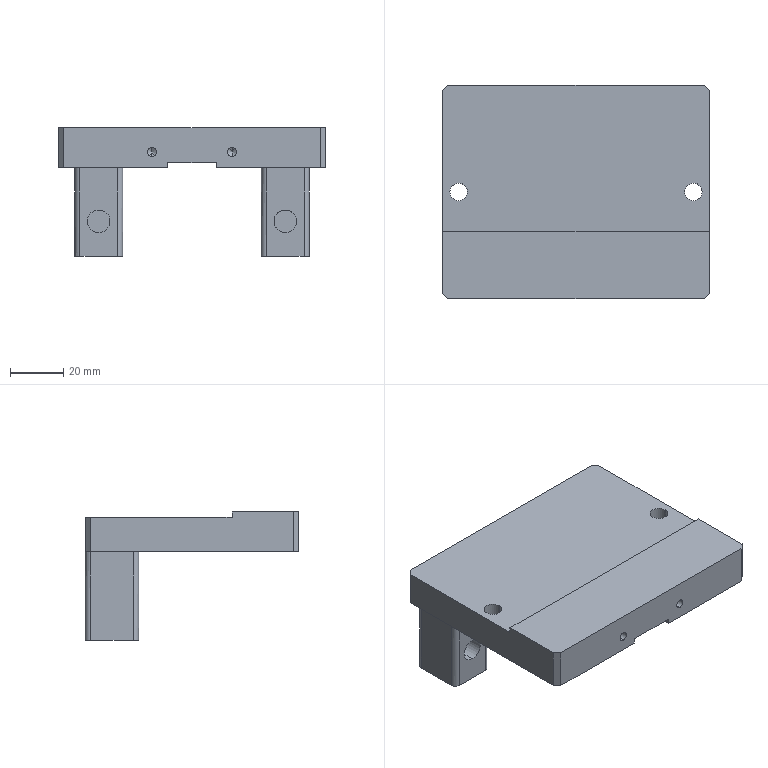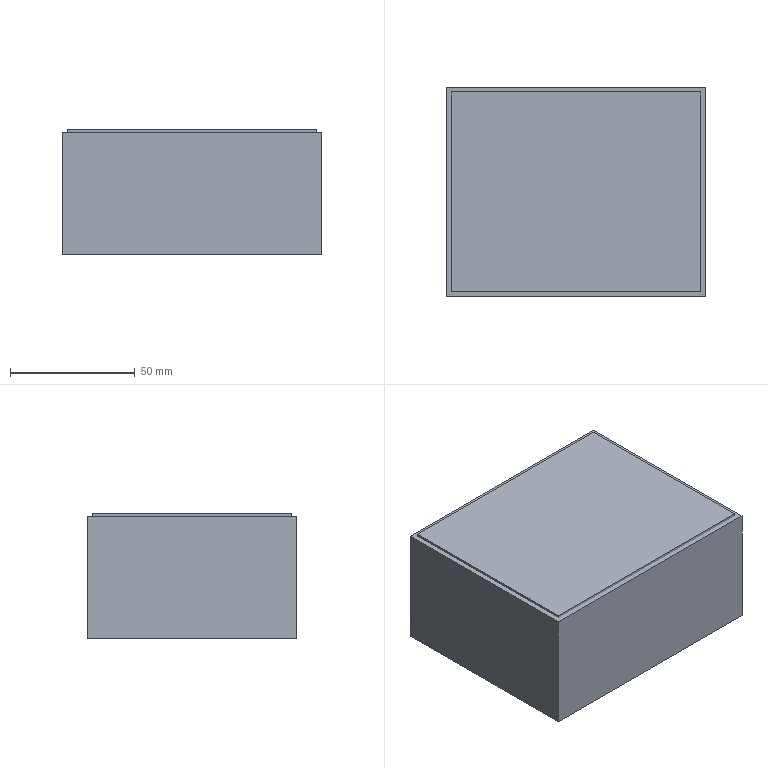CAM job | NX | 3-axis milling, drilling | part box 100 x 80 x 48 mm | stock box 104 x 84 x 50 mm
Tools:
number,name,description,diameter,corner_radius,flute_length,length,flutes
19,D80,Milling Tool-5 Parameters,80.0,0.0,50.0,75.0,2
15,D10,Milling Tool-5 Parameters,10.0,0.0,50.0,75.0,2
14,D10JING,Milling Tool-5 Parameters,10.0,0.0,50.0,75.0,2
12,D6,Milling Tool-5 Parameters,6.0,0.0,50.0,75.0,2
1,D6A45,Milling Tool-5 Parameters,6.0,0.0,50.0,75.0,2
9,6.6ZT,Drilling Tool,6.6,0.0,35.0,50.0,2
2,2.5ZT,Drilling Tool,2.0,0.0,35.0,50.0,2
Operations:
program,operation,operation_type,tool,method,geometry_group,spindle_rpm,surface_speed,feed_per_tooth,feed_cut,feed_plunge,cut_length_mm,path_length_mm,cut_time_min,machine_time_min
1,FLOOR_WALL,VolumeBased25DMillingOperation,D80,METHOD,A,6500.0,1633.0,0.1154,1500.0,100.0,615.997,669.997,0.4107,0.4161
1,ZLEVEL_PROFILE,ZLevelMilling,D10,METHOD,A,9500.0,298.0,0.1579,3000.0,1000.0,8183.565,8260.565,2.76,2.767
1,FLOOR_WALL_1,VolumeBased25DMillingOperation,D6,METHOD,A,9500.0,179.0,0.1053,2000.0,100.0,5811.853,5960.05,2.906,2.921
1,FLOOR_WALL_1_COPY_COPY_1,VolumeBased25DMillingOperation,D6,METHOD,A,9500.0,179.0,0.0632,1200.0,100.0,2006.367,2123.091,1.672,1.684
1,ZLEVEL_PROFILE_1,ZLevelMilling,D10JING,METHOD,A,9500.0,298.0,0.0789,1500.0,1000.0,395.068,492.068,0.2647,0.2744
1,PLANAR_MILL_COPY,PlanarMilling,D6A45,METHOD,A,9500.0,179.0,0.0658,1250.0,100.0,258.406,317.406,0.2067,0.2126
1,PLANAR_MILL_COPY_COPY,PlanarMilling,D6A45,METHOD,A,9500.0,179.0,0.0658,1250.0,100.0,253.964,639.105,0.2032,0.2417
2,FLOOR_WALL_COPY,VolumeBased25DMillingOperation,D80,METHOD,B,6500.0,1633.0,0.1154,1500.0,100.0,1199.994,1498.087,0.8,0.8298
2,FLOOR_WALL_1_COPY,VolumeBased25DMillingOperation,D10,METHOD,B,9500.0,298.0,0.1842,3500.0,100.0,53222.042,54526.332,15.206,15.337
2,FLOOR_WALL_1_COPY_COPY,VolumeBased25DMillingOperation,D10,METHOD,B,9500.0,298.0,0.1842,3500.0,100.0,406.008,534.897,0.116,0.1289
2,FLOOR_WALL_1_COPY_COPY_1_COPY_COPY_1,VolumeBased25DMillingOperation,D10JING,METHOD,B,9500.0,179.0,0.0632,1200.0,100.0,385.968,722.215,0.3216,0.3553
2,ZLEVEL_PROFILE_1_COPY,ZLevelMilling,D10JING,METHOD,B,9500.0,298.0,0.0789,1500.0,1000.0,229.809,552.805,0.1559,0.1882
2,FLOOR_WALL_1_COPY_COPY_1_COPY,VolumeBased25DMillingOperation,D10JING,METHOD,B,9500.0,179.0,0.0632,1200.0,100.0,1860.732,3343.881,1.551,1.699
2,FLOOR_WALL_1_COPY_COPY_1_COPY_COPY,VolumeBased25DMillingOperation,D10JING,METHOD,B,9500.0,179.0,0.0632,1200.0,100.0,482.104,613.208,0.4018,0.4149
2,HOLE_MILLING,CylinderMilling,D6,METHOD,B,9500.0,179.0,0.0789,1500.0,100.0,429.63,782.23,0.2864,0.3217
2,DRILLING,Operation,D6A45,METHOD,B,9500.0,179.0,0.0132,250.0,0.0,20.0,345.051,0.08,0.1125
2,DRILLING_COPY_COPY,Operation,6.6ZT,METHOD,B,2000.0,34.0,0.075,300.0,0.0,38.966,294.983,0.1299,0.1555
2,DRILLING_COPY_COPY_COPY,Operation,2.5ZT,METHOD,B,2000.0,12.0,0.025,100.0,0.0,33.753,263.806,0.3375,0.3605
2,PLANAR_MILL_COPY_COPY_1,PlanarMilling,D6A45,METHOD,B,9500.0,179.0,0.0658,1250.0,100.0,166.631,364.86,0.1333,0.1531
2,PLANAR_MILL_COPY_COPY_COPY,PlanarMilling,D6A45,METHOD,B,9500.0,179.0,0.0658,1250.0,100.0,529.377,1223.507,0.4235,0.4929
2,FLOOR_WALL_1_COPY_COPY_1_COPY_COPY_COPY,VolumeBased25DMillingOperation,D6,METHOD,B,9500.0,179.0,0.0632,1200.0,100.0,186.456,322.168,0.1554,0.169